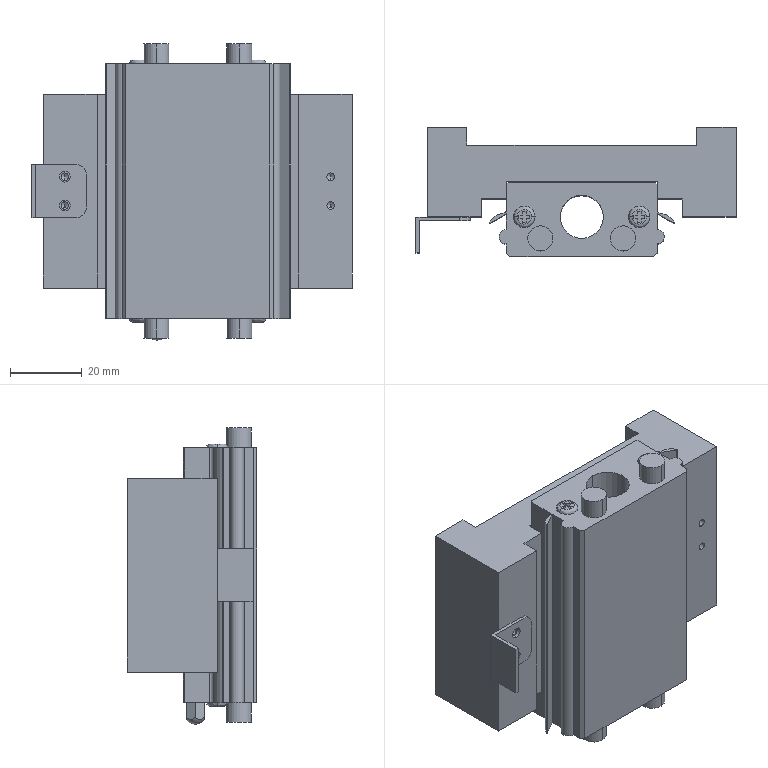Part | SolidWorks | features BaseBody 1 | 1 solid | 279 faces | box 89.2 x 36 x 82.5 mm | volume 126325 mm3 | plane 177 | cylinder 76 | cone 16 | spline 8 | torus 2 | commonest cylinder face diameters 2.113 x8 4.134 x8 5 x8 7 x8 9 x8 9.5 x8